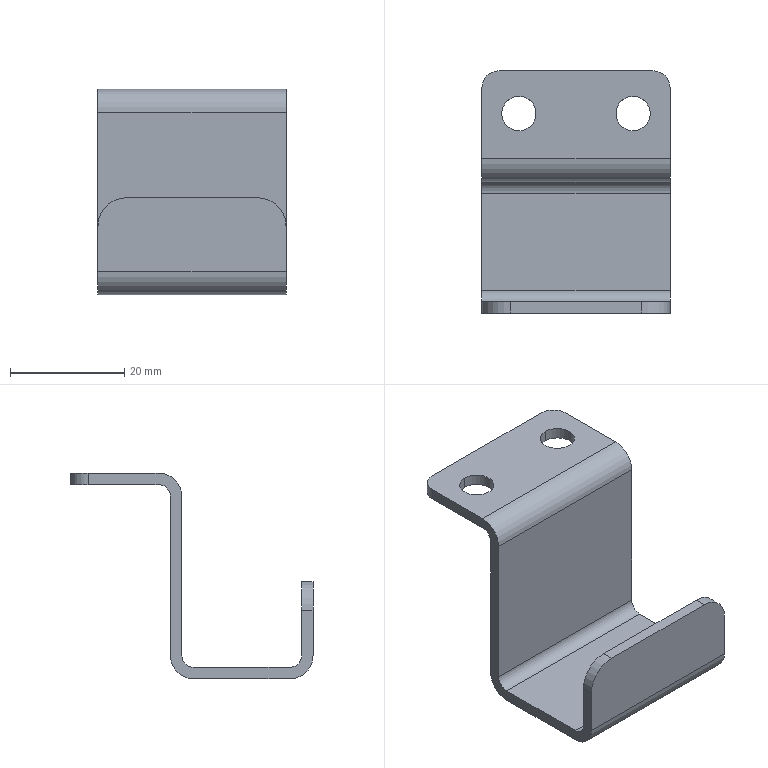Part | NX | features solid 2 | 1 solid | 26 faces | box 33 x 42.445 x 36 mm | volume 5638 mm3 | cylinder 14 | plane 12 | commonest cylinder face diameters 6 x6 4 x3 8 x3 10 x2
STEP:
#1=CARTESIAN_POINT('',(-461.,-1639.945,294.));
#2=VERTEX_POINT('',#1);
#3=CARTESIAN_POINT('',(-461.,-1637.945,296.));
#4=VERTEX_POINT('',#3);
#5=CARTESIAN_POINT('',(-461.,-1637.945,294.));
#6=DIRECTION('',(-1.,0.,0.));
#7=DIRECTION('',(0.,-1.,0.));
#8=AXIS2_PLACEMENT_3D('',#5,#6,#7);
#9=CIRCLE('',#8,2.);
#10=EDGE_CURVE('',#2,#4,#9,.T.);
#11=ORIENTED_EDGE('',*,*,#10,.F.);
#12=CARTESIAN_POINT('',(-494.,-1639.945,294.));
#13=VERTEX_POINT('',#12);
#14=CARTESIAN_POINT('',(-494.,-1639.945,294.));
#15=DIRECTION('',(1.,0.,0.));
#16=VECTOR('',#15,1000.);
#17=LINE('',#14,#16);
#18=EDGE_CURVE('',#13,#2,#17,.T.);
#19=ORIENTED_EDGE('',*,*,#18,.F.);
#20=CARTESIAN_POINT('',(-494.,-1637.945,296.));
#21=VERTEX_POINT('',#20);
#22=CARTESIAN_POINT('',(-494.,-1637.945,294.));
#23=DIRECTION('',(-1.,0.,0.));
#24=DIRECTION('',(0.,-1.,0.));
#25=AXIS2_PLACEMENT_3D('',#22,#23,#24);
#26=CIRCLE('',#25,2.);
#27=EDGE_CURVE('',#13,#21,#26,.T.);
#28=ORIENTED_EDGE('',*,*,#27,.T.);
#29=CARTESIAN_POINT('',(-494.,-1637.945,296.));
#30=DIRECTION('',(1.,0.,0.));
#31=VECTOR('',#30,1000.);
#32=LINE('',#29,#31);
#33=EDGE_CURVE('',#21,#4,#32,.T.);
#34=ORIENTED_EDGE('',*,*,#33,.T.);
#35=EDGE_LOOP('',(#11,#19,#28,#34));
#36=FACE_BOUND('',#35,.T.);
#37=CARTESIAN_POINT('',(-461.,-1637.945,294.));
#38=DIRECTION('',(-1.,0.,0.));
#39=DIRECTION('',(0.,1.,0.));
#40=AXIS2_PLACEMENT_3D('',#37,#38,#39);
#41=CYLINDRICAL_SURFACE('',#40,2.);
#42=ADVANCED_FACE('',(#36),#41,.F.);
#43=CARTESIAN_POINT('',(-461.,-1641.945,294.));
#44=VERTEX_POINT('',#43);
#45=CARTESIAN_POINT('',(-461.,-1637.945,298.));
#46=VERTEX_POINT('',#45);
#47=CARTESIAN_POINT('',(-461.,-1637.945,294.));
#48=DIRECTION('',(-1.,0.,0.));
#49=DIRECTION('',(0.,1.,0.));
#50=AXIS2_PLACEMENT_3D('',#47,#48,#49);
#51=CIRCLE('',#50,4.);
#52=EDGE_CURVE('',#44,#46,#51,.T.);
#53=ORIENTED_EDGE('',*,*,#52,.T.);
#54=CARTESIAN_POINT('',(-494.,-1637.945,298.));
#55=VERTEX_POINT('',#54);
#56=CARTESIAN_POINT('',(-494.,-1637.945,298.));
#57=DIRECTION('',(1.,0.,0.));
#58=VECTOR('',#57,1000.);
#59=LINE('',#56,#58);
#60=EDGE_CURVE('',#55,#46,#59,.T.);
#61=ORIENTED_EDGE('',*,*,#60,.F.);
#62=CARTESIAN_POINT('',(-494.,-1641.945,294.));
#63=VERTEX_POINT('',#62);
#64=CARTESIAN_POINT('',(-494.,-1637.945,294.));
#65=DIRECTION('',(-1.,0.,0.));
#66=DIRECTION('',(0.,1.,0.));
#67=AXIS2_PLACEMENT_3D('',#64,#65,#66);
#68=CIRCLE('',#67,4.);
#69=EDGE_CURVE('',#63,#55,#68,.T.);
#70=ORIENTED_EDGE('',*,*,#69,.F.);
#71=CARTESIAN_POINT('',(-494.,-1641.945,294.));
#72=DIRECTION('',(1.,0.,0.));
#73=VECTOR('',#72,1000.);
#74=LINE('',#71,#73);
#75=EDGE_CURVE('',#63,#44,#74,.T.);
#76=ORIENTED_EDGE('',*,*,#75,.T.);
#77=EDGE_LOOP('',(#53,#61,#70,#76));
#78=FACE_BOUND('',#77,.T.);
#79=CARTESIAN_POINT('',(-461.,-1637.945,294.));
#80=DIRECTION('',(-1.,0.,0.));
#81=DIRECTION('',(0.,1.,0.));
#82=AXIS2_PLACEMENT_3D('',#79,#80,#81);
#83=CYLINDRICAL_SURFACE('',#82,4.);
#84=ADVANCED_FACE('',(#78),#83,.T.);
#85=CARTESIAN_POINT('',(-467.5,-1627.,296.));
#86=VERTEX_POINT('',#85);
#87=CARTESIAN_POINT('',(-467.5,-1633.,296.));
#88=VERTEX_POINT('',#87);
#89=CARTESIAN_POINT('',(-467.5,-1630.,296.));
#90=DIRECTION('',(0.,0.,-1.));
#91=DIRECTION('',(0.,-1.,0.));
#92=AXIS2_PLACEMENT_3D('',#89,#90,#91);
#93=CIRCLE('',#92,3.);
#94=EDGE_CURVE('',#86,#88,#93,.T.);
#95=ORIENTED_EDGE('',*,*,#94,.F.);
#96=CARTESIAN_POINT('',(-467.5,-1630.,296.));
#97=DIRECTION('',(0.,0.,-1.));
#98=DIRECTION('',(0.,-1.,0.));
#99=AXIS2_PLACEMENT_3D('',#96,#97,#98);
#100=CIRCLE('',#99,3.);
#101=EDGE_CURVE('',#88,#86,#100,.T.);
#102=ORIENTED_EDGE('',*,*,#101,.F.);
#103=EDGE_LOOP('',(#95,#102));
#104=FACE_BOUND('',#103,.T.);
#105=CARTESIAN_POINT('',(-487.5,-1627.,296.));
#106=VERTEX_POINT('',#105);
#107=CARTESIAN_POINT('',(-487.5,-1633.,296.));
#108=VERTEX_POINT('',#107);
#109=CARTESIAN_POINT('',(-487.5,-1630.,296.));
#110=DIRECTION('',(0.,0.,-1.));
#111=DIRECTION('',(0.,-1.,0.));
#112=AXIS2_PLACEMENT_3D('',#109,#110,#111);
#113=CIRCLE('',#112,3.);
#114=EDGE_CURVE('',#106,#108,#113,.T.);
#115=ORIENTED_EDGE('',*,*,#114,.F.);
#116=CARTESIAN_POINT('',(-487.5,-1630.,296.));
#117=DIRECTION('',(0.,0.,-1.));
#118=DIRECTION('',(0.,-1.,0.));
#119=AXIS2_PLACEMENT_3D('',#116,#117,#118);
#120=CIRCLE('',#119,3.);
#121=EDGE_CURVE('',#108,#106,#120,.T.);
#122=ORIENTED_EDGE('',*,*,#121,.F.);
#123=EDGE_LOOP('',(#115,#122));
#124=FACE_BOUND('',#123,.T.);
#125=ORIENTED_EDGE('',*,*,#33,.F.);
#126=CARTESIAN_POINT('',(-494.,-1625.5,296.));
#127=VERTEX_POINT('',#126);
#128=CARTESIAN_POINT('',(-494.,-1622.5,296.));
#129=DIRECTION('',(0.,1.,0.));
#130=VECTOR('',#129,1000.);
#131=LINE('',#128,#130);
#132=EDGE_CURVE('',#21,#127,#131,.T.);
#133=ORIENTED_EDGE('',*,*,#132,.T.);
#134=CARTESIAN_POINT('',(-491.,-1622.5,296.));
#135=VERTEX_POINT('',#134);
#136=CARTESIAN_POINT('',(-491.,-1625.5,296.));
#137=DIRECTION('',(0.,0.,-1.));
#138=DIRECTION('',(0.,-1.,0.));
#139=AXIS2_PLACEMENT_3D('',#136,#137,#138);
#140=CIRCLE('',#139,3.);
#141=EDGE_CURVE('',#127,#135,#140,.T.);
#142=ORIENTED_EDGE('',*,*,#141,.T.);
#143=CARTESIAN_POINT('',(-464.,-1622.5,296.));
#144=VERTEX_POINT('',#143);
#145=CARTESIAN_POINT('',(-494.,-1622.5,296.));
#146=DIRECTION('',(1.,0.,0.));
#147=VECTOR('',#146,1000.);
#148=LINE('',#145,#147);
#149=EDGE_CURVE('',#135,#144,#148,.T.);
#150=ORIENTED_EDGE('',*,*,#149,.T.);
#151=CARTESIAN_POINT('',(-461.,-1625.5,296.));
#152=VERTEX_POINT('',#151);
#153=CARTESIAN_POINT('',(-464.,-1625.5,296.));
#154=DIRECTION('',(0.,0.,-1.));
#155=DIRECTION('',(0.,-1.,0.));
#156=AXIS2_PLACEMENT_3D('',#153,#154,#155);
#157=CIRCLE('',#156,3.);
#158=EDGE_CURVE('',#144,#152,#157,.T.);
#159=ORIENTED_EDGE('',*,*,#158,.T.);
#160=CARTESIAN_POINT('',(-461.,-1622.5,296.));
#161=DIRECTION('',(0.,1.,0.));
#162=VECTOR('',#161,1000.);
#163=LINE('',#160,#162);
#164=EDGE_CURVE('',#4,#152,#163,.T.);
#165=ORIENTED_EDGE('',*,*,#164,.F.);
#166=EDGE_LOOP('',(#125,#133,#142,#150,#159,#165));
#167=FACE_BOUND('',#166,.T.);
#168=CARTESIAN_POINT('',(-494.,-1622.5,296.));
#169=DIRECTION('',(0.,0.,-1.));
#170=DIRECTION('',(0.,-1.,0.));
#171=AXIS2_PLACEMENT_3D('',#168,#169,#170);
#172=PLANE('',#171);
#173=ADVANCED_FACE('',(#104,#124,#167),#172,.T.);
#174=CARTESIAN_POINT('',(-467.5,-1627.,298.));
#175=VERTEX_POINT('',#174);
#176=CARTESIAN_POINT('',(-467.5,-1633.,298.));
#177=VERTEX_POINT('',#176);
#178=CARTESIAN_POINT('',(-467.5,-1630.,298.));
#179=DIRECTION('',(0.,0.,1.));
#180=DIRECTION('',(1.,0.,0.));
#181=AXIS2_PLACEMENT_3D('',#178,#179,#180);
#182=CIRCLE('',#181,3.);
#183=EDGE_CURVE('',#175,#177,#182,.T.);
#184=ORIENTED_EDGE('',*,*,#183,.F.);
#185=CARTESIAN_POINT('',(-467.5,-1630.,298.));
#186=DIRECTION('',(0.,0.,1.));
#187=DIRECTION('',(1.,0.,0.));
#188=AXIS2_PLACEMENT_3D('',#185,#186,#187);
#189=CIRCLE('',#188,3.);
#190=EDGE_CURVE('',#177,#175,#189,.T.);
#191=ORIENTED_EDGE('',*,*,#190,.F.);
#192=EDGE_LOOP('',(#184,#191));
#193=FACE_BOUND('',#192,.T.);
#194=CARTESIAN_POINT('',(-487.5,-1627.,298.));
#195=VERTEX_POINT('',#194);
#196=CARTESIAN_POINT('',(-487.5,-1633.,298.));
#197=VERTEX_POINT('',#196);
#198=CARTESIAN_POINT('',(-487.5,-1630.,298.));
#199=DIRECTION('',(0.,0.,1.));
#200=DIRECTION('',(1.,0.,0.));
#201=AXIS2_PLACEMENT_3D('',#198,#199,#200);
#202=CIRCLE('',#201,3.);
#203=EDGE_CURVE('',#195,#197,#202,.T.);
#204=ORIENTED_EDGE('',*,*,#203,.F.);
#205=CARTESIAN_POINT('',(-487.5,-1630.,298.));
#206=DIRECTION('',(0.,0.,1.));
#207=DIRECTION('',(1.,0.,0.));
#208=AXIS2_PLACEMENT_3D('',#205,#206,#207);
#209=CIRCLE('',#208,3.);
#210=EDGE_CURVE('',#197,#195,#209,.T.);
#211=ORIENTED_EDGE('',*,*,#210,.F.);
#212=EDGE_LOOP('',(#204,#211));
#213=FACE_BOUND('',#212,.T.);
#214=CARTESIAN_POINT('',(-494.,-1625.5,298.));
#215=VERTEX_POINT('',#214);
#216=CARTESIAN_POINT('',(-494.,-1622.5,298.));
#217=DIRECTION('',(0.,1.,0.));
#218=VECTOR('',#217,1000.);
#219=LINE('',#216,#218);
#220=EDGE_CURVE('',#55,#215,#219,.T.);
#221=ORIENTED_EDGE('',*,*,#220,.F.);
#222=ORIENTED_EDGE('',*,*,#60,.T.);
#223=CARTESIAN_POINT('',(-461.,-1625.5,298.));
#224=VERTEX_POINT('',#223);
#225=CARTESIAN_POINT('',(-461.,-1622.5,298.));
#226=DIRECTION('',(0.,1.,0.));
#227=VECTOR('',#226,1000.);
#228=LINE('',#225,#227);
#229=EDGE_CURVE('',#46,#224,#228,.T.);
#230=ORIENTED_EDGE('',*,*,#229,.T.);
#231=CARTESIAN_POINT('',(-464.,-1622.5,298.));
#232=VERTEX_POINT('',#231);
#233=CARTESIAN_POINT('',(-464.,-1625.5,298.));
#234=DIRECTION('',(0.,0.,1.));
#235=DIRECTION('',(0.,-1.,0.));
#236=AXIS2_PLACEMENT_3D('',#233,#234,#235);
#237=CIRCLE('',#236,3.);
#238=EDGE_CURVE('',#224,#232,#237,.T.);
#239=ORIENTED_EDGE('',*,*,#238,.T.);
#240=CARTESIAN_POINT('',(-491.,-1622.5,298.));
#241=VERTEX_POINT('',#240);
#242=CARTESIAN_POINT('',(-494.,-1622.5,298.));
#243=DIRECTION('',(1.,0.,0.));
#244=VECTOR('',#243,1000.);
#245=LINE('',#242,#244);
#246=EDGE_CURVE('',#241,#232,#245,.T.);
#247=ORIENTED_EDGE('',*,*,#246,.F.);
#248=CARTESIAN_POINT('',(-491.,-1625.5,298.));
#249=DIRECTION('',(0.,0.,1.));
#250=DIRECTION('',(0.,-1.,0.));
#251=AXIS2_PLACEMENT_3D('',#248,#249,#250);
#252=CIRCLE('',#251,3.);
#253=EDGE_CURVE('',#241,#215,#252,.T.);
#254=ORIENTED_EDGE('',*,*,#253,.T.);
#255=EDGE_LOOP('',(#221,#222,#230,#239,#247,#254));
#256=FACE_BOUND('',#255,.T.);
#257=CARTESIAN_POINT('',(-494.,-1622.5,298.));
#258=DIRECTION('',(0.,0.,-1.));
#259=DIRECTION('',(0.,-1.,0.));
#260=AXIS2_PLACEMENT_3D('',#257,#258,#259);
#261=PLANE('',#260);
#262=ADVANCED_FACE('',(#193,#213,#256),#261,.F.);
#263=ORIENTED_EDGE('',*,*,#141,.F.);
#264=CARTESIAN_POINT('',(-494.,-1625.5,319.));
#265=DIRECTION('',(0.,0.,-1.));
#266=VECTOR('',#265,1000.);
#267=LINE('',#264,#266);
#268=EDGE_CURVE('',#215,#127,#267,.T.);
#269=ORIENTED_EDGE('',*,*,#268,.F.);
#270=ORIENTED_EDGE('',*,*,#253,.F.);
#271=CARTESIAN_POINT('',(-491.,-1622.5,298.));
#272=DIRECTION('',(0.,0.,1.));
#273=VECTOR('',#272,1000.);
#274=LINE('',#271,#273);
#275=EDGE_CURVE('',#135,#241,#274,.T.);
#276=ORIENTED_EDGE('',*,*,#275,.F.);
#277=EDGE_LOOP('',(#263,#269,#270,#276));
#278=FACE_BOUND('',#277,.T.);
#279=CARTESIAN_POINT('',(-491.,-1625.5,298.));
#280=DIRECTION('',(0.,0.,1.));
#281=DIRECTION('',(0.,1.,0.));
#282=AXIS2_PLACEMENT_3D('',#279,#280,#281);
#283=CYLINDRICAL_SURFACE('',#282,3.);
#284=ADVANCED_FACE('',(#278),#283,.T.);
#285=CARTESIAN_POINT('',(-487.5,-1633.,231.532));
#286=DIRECTION('',(0.,0.,1.));
#287=VECTOR('',#286,1000.);
#288=LINE('',#285,#287);
#289=EDGE_CURVE('',#197,#108,#288,.F.);
#290=ORIENTED_EDGE('',*,*,#289,.T.);
#291=ORIENTED_EDGE('',*,*,#121,.T.);
#292=CARTESIAN_POINT('',(-487.5,-1627.,231.532));
#293=DIRECTION('',(0.,0.,1.));
#294=VECTOR('',#293,1000.);
#295=LINE('',#292,#294);
#296=EDGE_CURVE('',#106,#195,#295,.T.);
#297=ORIENTED_EDGE('',*,*,#296,.T.);
#298=ORIENTED_EDGE('',*,*,#203,.T.);
#299=EDGE_LOOP('',(#290,#291,#297,#298));
#300=FACE_BOUND('',#299,.T.);
#301=CARTESIAN_POINT('',(-487.5,-1630.,231.532));
#302=DIRECTION('',(0.,0.,1.));
#303=DIRECTION('',(0.,1.,0.));
#304=AXIS2_PLACEMENT_3D('',#301,#302,#303);
#305=CYLINDRICAL_SURFACE('',#304,3.);
#306=ADVANCED_FACE('',(#300),#305,.F.);
#307=CARTESIAN_POINT('',(-467.5,-1633.,231.532));
#308=DIRECTION('',(0.,0.,1.));
#309=VECTOR('',#308,1000.);
#310=LINE('',#307,#309);
#311=EDGE_CURVE('',#177,#88,#310,.F.);
#312=ORIENTED_EDGE('',*,*,#311,.T.);
#313=ORIENTED_EDGE('',*,*,#101,.T.);
#314=CARTESIAN_POINT('',(-467.5,-1627.,231.532));
#315=DIRECTION('',(0.,0.,1.));
#316=VECTOR('',#315,1000.);
#317=LINE('',#314,#316);
#318=EDGE_CURVE('',#86,#175,#317,.T.);
#319=ORIENTED_EDGE('',*,*,#318,.T.);
#320=ORIENTED_EDGE('',*,*,#183,.T.);
#321=EDGE_LOOP('',(#312,#313,#319,#320));
#322=FACE_BOUND('',#321,.T.);
#323=CARTESIAN_POINT('',(-467.5,-1630.,231.532));
#324=DIRECTION('',(0.,0.,1.));
#325=DIRECTION('',(0.,1.,0.));
#326=AXIS2_PLACEMENT_3D('',#323,#324,#325);
#327=CYLINDRICAL_SURFACE('',#326,3.);
#328=ADVANCED_FACE('',(#322),#327,.F.);
#329=ORIENTED_EDGE('',*,*,#158,.F.);
#330=CARTESIAN_POINT('',(-464.,-1622.5,298.));
#331=DIRECTION('',(0.,0.,-1.));
#332=VECTOR('',#331,1000.);
#333=LINE('',#330,#332);
#334=EDGE_CURVE('',#232,#144,#333,.T.);
#335=ORIENTED_EDGE('',*,*,#334,.F.);
#336=ORIENTED_EDGE('',*,*,#238,.F.);
#337=CARTESIAN_POINT('',(-461.,-1625.5,317.));
#338=DIRECTION('',(0.,0.,1.));
#339=VECTOR('',#338,1000.);
#340=LINE('',#337,#339);
#341=EDGE_CURVE('',#152,#224,#340,.T.);
#342=ORIENTED_EDGE('',*,*,#341,.F.);
#343=EDGE_LOOP('',(#329,#335,#336,#342));
#344=FACE_BOUND('',#343,.T.);
#345=CARTESIAN_POINT('',(-464.,-1625.5,317.));
#346=DIRECTION('',(0.,0.,1.));
#347=DIRECTION('',(0.,1.,0.));
#348=AXIS2_PLACEMENT_3D('',#345,#346,#347);
#349=CYLINDRICAL_SURFACE('',#348,3.);
#350=ADVANCED_FACE('',(#344),#349,.T.);
#351=ORIENTED_EDGE('',*,*,#246,.T.);
#352=ORIENTED_EDGE('',*,*,#334,.T.);
#353=ORIENTED_EDGE('',*,*,#149,.F.);
#354=ORIENTED_EDGE('',*,*,#275,.T.);
#355=EDGE_LOOP('',(#351,#352,#353,#354));
#356=FACE_BOUND('',#355,.T.);
#357=CARTESIAN_POINT('',(-494.,-1622.5,298.));
#358=DIRECTION('',(0.,1.,0.));
#359=DIRECTION('',(1.,0.,0.));
#360=AXIS2_PLACEMENT_3D('',#357,#358,#359);
#361=PLANE('',#360);
#362=ADVANCED_FACE('',(#356),#361,.T.);
#363=CARTESIAN_POINT('',(-489.,-1664.945,279.));
#364=VERTEX_POINT('',#363);
#365=CARTESIAN_POINT('',(-494.,-1664.945,274.));
#366=VERTEX_POINT('',#365);
#367=CARTESIAN_POINT('',(-489.,-1664.945,274.));
#368=DIRECTION('',(0.,-1.,0.));
#369=DIRECTION('',(1.,0.,0.));
#370=AXIS2_PLACEMENT_3D('',#367,#368,#369);
#371=CIRCLE('',#370,5.);
#372=EDGE_CURVE('',#364,#366,#371,.T.);
#373=ORIENTED_EDGE('',*,*,#372,.F.);
#374=CARTESIAN_POINT('',(-489.,-1662.945,279.));
#375=VERTEX_POINT('',#374);
#376=CARTESIAN_POINT('',(-489.,-1662.945,279.));
#377=DIRECTION('',(0.,-1.,0.));
#378=VECTOR('',#377,1000.);
#379=LINE('',#376,#378);
#380=EDGE_CURVE('',#375,#364,#379,.T.);
#381=ORIENTED_EDGE('',*,*,#380,.F.);
#382=CARTESIAN_POINT('',(-494.,-1662.945,274.));
#383=VERTEX_POINT('',#382);
#384=CARTESIAN_POINT('',(-489.,-1662.945,274.));
#385=DIRECTION('',(0.,1.,0.));
#386=DIRECTION('',(1.,0.,0.));
#387=AXIS2_PLACEMENT_3D('',#384,#385,#386);
#388=CIRCLE('',#387,5.);
#389=EDGE_CURVE('',#383,#375,#388,.T.);
#390=ORIENTED_EDGE('',*,*,#389,.F.);
#391=CARTESIAN_POINT('',(-494.,-1662.945,274.));
#392=DIRECTION('',(0.,1.,0.));
#393=VECTOR('',#392,1000.);
#394=LINE('',#391,#393);
#395=EDGE_CURVE('',#366,#383,#394,.T.);
#396=ORIENTED_EDGE('',*,*,#395,.F.);
#397=EDGE_LOOP('',(#373,#381,#390,#396));
#398=FACE_BOUND('',#397,.T.);
#399=CARTESIAN_POINT('',(-489.,-1662.945,274.));
#400=DIRECTION('',(0.,-1.,0.));
#401=DIRECTION('',(1.,0.,0.));
#402=AXIS2_PLACEMENT_3D('',#399,#400,#401);
#403=CYLINDRICAL_SURFACE('',#402,5.);
#404=ADVANCED_FACE('',(#398),#403,.T.);
#405=CARTESIAN_POINT('',(-461.,-1664.945,274.));
#406=VERTEX_POINT('',#405);
#407=CARTESIAN_POINT('',(-466.,-1664.945,279.));
#408=VERTEX_POINT('',#407);
#409=CARTESIAN_POINT('',(-466.,-1664.945,274.));
#410=DIRECTION('',(0.,-1.,0.));
#411=DIRECTION('',(1.,0.,0.));
#412=AXIS2_PLACEMENT_3D('',#409,#410,#411);
#413=CIRCLE('',#412,5.);
#414=EDGE_CURVE('',#406,#408,#413,.T.);
#415=ORIENTED_EDGE('',*,*,#414,.F.);
#416=CARTESIAN_POINT('',(-461.,-1662.945,274.));
#417=VERTEX_POINT('',#416);
#418=CARTESIAN_POINT('',(-461.,-1660.945,274.));
#419=DIRECTION('',(0.,-1.,0.));
#420=VECTOR('',#419,1000.);
#421=LINE('',#418,#420);
#422=EDGE_CURVE('',#417,#406,#421,.T.);
#423=ORIENTED_EDGE('',*,*,#422,.F.);
#424=CARTESIAN_POINT('',(-466.,-1662.945,279.));
#425=VERTEX_POINT('',#424);
#426=CARTESIAN_POINT('',(-466.,-1662.945,274.));
#427=DIRECTION('',(0.,1.,0.));
#428=DIRECTION('',(1.,0.,0.));
#429=AXIS2_PLACEMENT_3D('',#426,#427,#428);
#430=CIRCLE('',#429,5.);
#431=EDGE_CURVE('',#425,#417,#430,.T.);
#432=ORIENTED_EDGE('',*,*,#431,.F.);
#433=CARTESIAN_POINT('',(-466.,-1662.945,279.));
#434=DIRECTION('',(0.,1.,0.));
#435=VECTOR('',#434,1000.);
#436=LINE('',#433,#435);
#437=EDGE_CURVE('',#408,#425,#436,.T.);
#438=ORIENTED_EDGE('',*,*,#437,.F.);
#439=EDGE_LOOP('',(#415,#423,#432,#438));
#440=FACE_BOUND('',#439,.T.);
#441=CARTESIAN_POINT('',(-466.,-1662.945,274.));
#442=DIRECTION('',(0.,-1.,0.));
#443=DIRECTION('',(1.,0.,0.));
#444=AXIS2_PLACEMENT_3D('',#441,#442,#443);
#445=CYLINDRICAL_SURFACE('',#444,5.);
#446=ADVANCED_FACE('',(#440),#445,.T.);
#447=CARTESIAN_POINT('',(-461.,-1643.945,262.));
#448=VERTEX_POINT('',#447);
#449=CARTESIAN_POINT('',(-461.,-1639.945,266.));
#450=VERTEX_POINT('',#449);
#451=CARTESIAN_POINT('',(-461.,-1643.945,266.));
#452=DIRECTION('',(1.,0.,0.));
#453=DIRECTION('',(0.,1.,0.));
#454=AXIS2_PLACEMENT_3D('',#451,#452,#453);
#455=CIRCLE('',#454,4.);
#456=EDGE_CURVE('',#448,#450,#455,.T.);
#457=ORIENTED_EDGE('',*,*,#456,.F.);
#458=CARTESIAN_POINT('',(-494.,-1643.945,262.));
#459=VERTEX_POINT('',#458);
#460=CARTESIAN_POINT('',(-494.,-1643.945,262.));
#461=DIRECTION('',(1.,0.,0.));
#462=VECTOR('',#461,1000.);
#463=LINE('',#460,#462);
#464=EDGE_CURVE('',#459,#448,#463,.T.);
#465=ORIENTED_EDGE('',*,*,#464,.F.);
#466=CARTESIAN_POINT('',(-494.,-1639.945,266.));
#467=VERTEX_POINT('',#466);
#468=CARTESIAN_POINT('',(-494.,-1643.945,266.));
#469=DIRECTION('',(1.,0.,0.));
#470=DIRECTION('',(0.,1.,0.));
#471=AXIS2_PLACEMENT_3D('',#468,#469,#470);
#472=CIRCLE('',#471,4.);
#473=EDGE_CURVE('',#459,#467,#472,.T.);
#474=ORIENTED_EDGE('',*,*,#473,.T.);
#475=CARTESIAN_POINT('',(-494.,-1639.945,266.));
#476=DIRECTION('',(1.,0.,0.));
#477=VECTOR('',#476,1000.);
#478=LINE('',#475,#477);
#479=EDGE_CURVE('',#467,#450,#478,.T.);
#480=ORIENTED_EDGE('',*,*,#479,.T.);
#481=EDGE_LOOP('',(#457,#465,#474,#480));
#482=FACE_BOUND('',#481,.T.);
#483=CARTESIAN_POINT('',(-494.,-1643.945,266.));
#484=DIRECTION('',(1.,0.,0.));
#485=DIRECTION('',(0.,1.,0.));
#486=AXIS2_PLACEMENT_3D('',#483,#484,#485);
#487=CYLINDRICAL_SURFACE('',#486,4.);
#488=ADVANCED_FACE('',(#482),#487,.T.);
#489=CARTESIAN_POINT('',(-461.,-1660.945,262.));
#490=VERTEX_POINT('',#489);
#491=CARTESIAN_POINT('',(-461.,-1641.945,262.));
#492=DIRECTION('',(0.,1.,0.));
#493=VECTOR('',#492,1000.);
#494=LINE('',#491,#493);
#495=EDGE_CURVE('',#490,#448,#494,.T.);
#496=ORIENTED_EDGE('',*,*,#495,.F.);
#497=CARTESIAN_POINT('',(-494.,-1660.945,262.));
#498=VERTEX_POINT('',#497);
#499=CARTESIAN_POINT('',(-494.,-1660.945,262.));
#500=DIRECTION('',(1.,0.,0.));
#501=VECTOR('',#500,1000.);
#502=LINE('',#499,#501);
#503=EDGE_CURVE('',#498,#490,#502,.T.);
#504=ORIENTED_EDGE('',*,*,#503,.F.);
#505=CARTESIAN_POINT('',(-494.,-1641.945,262.));
#506=DIRECTION('',(0.,1.,0.));
#507=VECTOR('',#506,1000.);
#508=LINE('',#505,#507);
#509=EDGE_CURVE('',#498,#459,#508,.T.);
#510=ORIENTED_EDGE('',*,*,#509,.T.);
#511=ORIENTED_EDGE('',*,*,#464,.T.);
#512=EDGE_LOOP('',(#496,#504,#510,#511));
#513=FACE_BOUND('',#512,.T.);
#514=CARTESIAN_POINT('',(-494.,-1641.945,262.));
#515=DIRECTION('',(0.,0.,-1.));
#516=DIRECTION('',(0.,-1.,0.));
#517=AXIS2_PLACEMENT_3D('',#514,#515,#516);
#518=PLANE('',#517);
#519=ADVANCED_FACE('',(#513),#518,.T.);
#520=CARTESIAN_POINT('',(-461.,-1664.945,266.));
#521=VERTEX_POINT('',#520);
#522=CARTESIAN_POINT('',(-461.,-1660.945,266.));
#523=DIRECTION('',(1.,0.,0.));
#524=DIRECTION('',(0.,1.,0.));
#525=AXIS2_PLACEMENT_3D('',#522,#523,#524);
#526=CIRCLE('',#525,4.);
#527=EDGE_CURVE('',#521,#490,#526,.T.);
#528=ORIENTED_EDGE('',*,*,#527,.F.);
#529=CARTESIAN_POINT('',(-494.,-1664.945,266.));
#530=VERTEX_POINT('',#529);
#531=CARTESIAN_POINT('',(-494.,-1664.945,266.));
#532=DIRECTION('',(1.,0.,0.));
#533=VECTOR('',#532,1000.);
#534=LINE('',#531,#533);
#535=EDGE_CURVE('',#530,#521,#534,.T.);
#536=ORIENTED_EDGE('',*,*,#535,.F.);
#537=CARTESIAN_POINT('',(-494.,-1660.945,266.));
#538=DIRECTION('',(1.,0.,0.));
#539=DIRECTION('',(0.,1.,0.));
#540=AXIS2_PLACEMENT_3D('',#537,#538,#539);
#541=CIRCLE('',#540,4.);
#542=EDGE_CURVE('',#530,#498,#541,.T.);
#543=ORIENTED_EDGE('',*,*,#542,.T.);
#544=ORIENTED_EDGE('',*,*,#503,.T.);
#545=EDGE_LOOP('',(#528,#536,#543,#544));
#546=FACE_BOUND('',#545,.T.);
#547=CARTESIAN_POINT('',(-494.,-1660.945,266.));
#548=DIRECTION('',(1.,0.,0.));
#549=DIRECTION('',(0.,1.,0.));
#550=AXIS2_PLACEMENT_3D('',#547,#548,#549);
#551=CYLINDRICAL_SURFACE('',#550,4.);
#552=ADVANCED_FACE('',(#546),#551,.T.);
#553=CARTESIAN_POINT('',(-461.,-1664.945,264.));
#554=DIRECTION('',(0.,0.,-1.));
#555=VECTOR('',#554,1000.);
#556=LINE('',#553,#555);
#557=EDGE_CURVE('',#406,#521,#556,.T.);
#558=ORIENTED_EDGE('',*,*,#557,.F.);
#559=ORIENTED_EDGE('',*,*,#414,.T.);
#560=CARTESIAN_POINT('',(-494.,-1664.945,279.));
#561=DIRECTION('',(1.,0.,0.));
#562=VECTOR('',#561,1000.);
#563=LINE('',#560,#562);
#564=EDGE_CURVE('',#364,#408,#563,.T.);
#565=ORIENTED_EDGE('',*,*,#564,.F.);
#566=ORIENTED_EDGE('',*,*,#372,.T.);
#567=CARTESIAN_POINT('',(-494.,-1664.945,264.));
#568=DIRECTION('',(0.,0.,-1.));
#569=VECTOR('',#568,1000.);
#570=LINE('',#567,#569);
#571=EDGE_CURVE('',#366,#530,#570,.T.);
#572=ORIENTED_EDGE('',*,*,#571,.T.);
#573=ORIENTED_EDGE('',*,*,#535,.T.);
#574=EDGE_LOOP('',(#558,#559,#565,#566,#572,#573));
#575=FACE_BOUND('',#574,.T.);
#576=CARTESIAN_POINT('',(-494.,-1664.945,264.));
#577=DIRECTION('',(0.,-1.,0.));
#578=DIRECTION('',(0.,0.,-1.));
#579=AXIS2_PLACEMENT_3D('',#576,#577,#578);
#580=PLANE('',#579);
#581=ADVANCED_FACE('',(#575),#580,.T.);
#582=ORIENTED_EDGE('',*,*,#75,.F.);
#583=CARTESIAN_POINT('',(-494.,-1641.945,266.));
#584=VERTEX_POINT('',#583);
#585=CARTESIAN_POINT('',(-494.,-1641.945,314.));
#586=DIRECTION('',(0.,0.,1.));
#587=VECTOR('',#586,1000.);
#588=LINE('',#585,#587);
#589=EDGE_CURVE('',#584,#63,#588,.T.);
#590=ORIENTED_EDGE('',*,*,#589,.F.);
#591=CARTESIAN_POINT('',(-461.,-1641.945,266.));
#592=VERTEX_POINT('',#591);
#593=CARTESIAN_POINT('',(-494.,-1641.945,266.));
#594=DIRECTION('',(1.,0.,0.));
#595=VECTOR('',#594,1000.);
#596=LINE('',#593,#595);
#597=EDGE_CURVE('',#584,#592,#596,.T.);
#598=ORIENTED_EDGE('',*,*,#597,.T.);
#599=CARTESIAN_POINT('',(-461.,-1641.945,314.));
#600=DIRECTION('',(0.,0.,1.));
#601=VECTOR('',#600,1000.);
#602=LINE('',#599,#601);
#603=EDGE_CURVE('',#592,#44,#602,.T.);
#604=ORIENTED_EDGE('',*,*,#603,.T.);
#605=EDGE_LOOP('',(#582,#590,#598,#604));
#606=FACE_BOUND('',#605,.T.);
#607=CARTESIAN_POINT('',(-494.,-1641.945,314.));
#608=DIRECTION('',(0.,1.,0.));
#609=DIRECTION('',(1.,0.,0.));
#610=AXIS2_PLACEMENT_3D('',#607,#608,#609);
#611=PLANE('',#610);
#612=ADVANCED_FACE('',(#606),#611,.F.);
#613=CARTESIAN_POINT('',(-461.,-1643.945,264.));
#614=VERTEX_POINT('',#613);
#615=CARTESIAN_POINT('',(-461.,-1643.945,266.));
#616=DIRECTION('',(1.,0.,0.));
#617=DIRECTION('',(0.,-1.,0.));
#618=AXIS2_PLACEMENT_3D('',#615,#616,#617);
#619=CIRCLE('',#618,2.);
#620=EDGE_CURVE('',#614,#592,#619,.T.);
#621=ORIENTED_EDGE('',*,*,#620,.T.);
#622=ORIENTED_EDGE('',*,*,#597,.F.);
#623=CARTESIAN_POINT('',(-494.,-1643.945,264.));
#624=VERTEX_POINT('',#623);
#625=CARTESIAN_POINT('',(-494.,-1643.945,266.));
#626=DIRECTION('',(1.,0.,0.));
#627=DIRECTION('',(0.,-1.,0.));
#628=AXIS2_PLACEMENT_3D('',#625,#626,#627);
#629=CIRCLE('',#628,2.);
#630=EDGE_CURVE('',#624,#584,#629,.T.);
#631=ORIENTED_EDGE('',*,*,#630,.F.);
#632=CARTESIAN_POINT('',(-494.,-1643.945,264.));
#633=DIRECTION('',(1.,0.,0.));
#634=VECTOR('',#633,1000.);
#635=LINE('',#632,#634);
#636=EDGE_CURVE('',#624,#614,#635,.T.);
#637=ORIENTED_EDGE('',*,*,#636,.T.);
#638=EDGE_LOOP('',(#621,#622,#631,#637));
#639=FACE_BOUND('',#638,.T.);
#640=CARTESIAN_POINT('',(-494.,-1643.945,266.));
#641=DIRECTION('',(1.,0.,0.));
#642=DIRECTION('',(0.,1.,0.));
#643=AXIS2_PLACEMENT_3D('',#640,#641,#642);
#644=CYLINDRICAL_SURFACE('',#643,2.);
#645=ADVANCED_FACE('',(#639),#644,.F.);
#646=CARTESIAN_POINT('',(-461.,-1660.945,264.));
#647=VERTEX_POINT('',#646);
#648=CARTESIAN_POINT('',(-461.,-1641.945,264.));
#649=DIRECTION('',(0.,1.,0.));
#650=VECTOR('',#649,1000.);
#651=LINE('',#648,#650);
#652=EDGE_CURVE('',#647,#614,#651,.T.);
#653=ORIENTED_EDGE('',*,*,#652,.T.);
#654=ORIENTED_EDGE('',*,*,#636,.F.);
#655=CARTESIAN_POINT('',(-494.,-1660.945,264.));
#656=VERTEX_POINT('',#655);
#657=CARTESIAN_POINT('',(-494.,-1641.945,264.));
#658=DIRECTION('',(0.,1.,0.));
#659=VECTOR('',#658,1000.);
#660=LINE('',#657,#659);
#661=EDGE_CURVE('',#656,#624,#660,.T.);
#662=ORIENTED_EDGE('',*,*,#661,.F.);
#663=CARTESIAN_POINT('',(-494.,-1660.945,264.));
#664=DIRECTION('',(1.,0.,0.));
#665=VECTOR('',#664,1000.);
#666=LINE('',#663,#665);
#667=EDGE_CURVE('',#656,#647,#666,.T.);
#668=ORIENTED_EDGE('',*,*,#667,.T.);
#669=EDGE_LOOP('',(#653,#654,#662,#668));
#670=FACE_BOUND('',#669,.T.);
#671=CARTESIAN_POINT('',(-494.,-1641.945,264.));
#672=DIRECTION('',(0.,0.,-1.));
#673=DIRECTION('',(0.,-1.,0.));
#674=AXIS2_PLACEMENT_3D('',#671,#672,#673);
#675=PLANE('',#674);
#676=ADVANCED_FACE('',(#670),#675,.F.);
#677=CARTESIAN_POINT('',(-461.,-1662.945,266.));
#678=VERTEX_POINT('',#677);
#679=CARTESIAN_POINT('',(-461.,-1660.945,266.));
#680=DIRECTION('',(1.,0.,0.));
#681=DIRECTION('',(0.,-1.,0.));
#682=AXIS2_PLACEMENT_3D('',#679,#680,#681);
#683=CIRCLE('',#682,2.);
#684=EDGE_CURVE('',#678,#647,#683,.T.);
#685=ORIENTED_EDGE('',*,*,#684,.T.);
#686=ORIENTED_EDGE('',*,*,#667,.F.);
#687=CARTESIAN_POINT('',(-494.,-1662.945,266.));
#688=VERTEX_POINT('',#687);
#689=CARTESIAN_POINT('',(-494.,-1660.945,266.));
#690=DIRECTION('',(1.,0.,0.));
#691=DIRECTION('',(0.,-1.,0.));
#692=AXIS2_PLACEMENT_3D('',#689,#690,#691);
#693=CIRCLE('',#692,2.);
#694=EDGE_CURVE('',#688,#656,#693,.T.);
#695=ORIENTED_EDGE('',*,*,#694,.F.);
#696=CARTESIAN_POINT('',(-494.,-1662.945,266.));
#697=DIRECTION('',(1.,0.,0.));
#698=VECTOR('',#697,1000.);
#699=LINE('',#696,#698);
#700=EDGE_CURVE('',#688,#678,#699,.T.);
#701=ORIENTED_EDGE('',*,*,#700,.T.);
#702=EDGE_LOOP('',(#685,#686,#695,#701));
#703=FACE_BOUND('',#702,.T.);
#704=CARTESIAN_POINT('',(-494.,-1660.945,266.));
#705=DIRECTION('',(1.,0.,0.));
#706=DIRECTION('',(0.,1.,0.));
#707=AXIS2_PLACEMENT_3D('',#704,#705,#706);
#708=CYLINDRICAL_SURFACE('',#707,2.);
#709=ADVANCED_FACE('',(#703),#708,.F.);
#710=CARTESIAN_POINT('',(-494.,-1662.945,279.));
#711=DIRECTION('',(1.,0.,0.));
#712=VECTOR('',#711,1000.);
#713=LINE('',#710,#712);
#714=EDGE_CURVE('',#375,#425,#713,.T.);
#715=ORIENTED_EDGE('',*,*,#714,.T.);
#716=ORIENTED_EDGE('',*,*,#431,.T.);
#717=CARTESIAN_POINT('',(-461.,-1662.945,264.));
#718=DIRECTION('',(0.,0.,-1.));
#719=VECTOR('',#718,1000.);
#720=LINE('',#717,#719);
#721=EDGE_CURVE('',#417,#678,#720,.T.);
#722=ORIENTED_EDGE('',*,*,#721,.T.);
#723=ORIENTED_EDGE('',*,*,#700,.F.);
#724=CARTESIAN_POINT('',(-494.,-1662.945,264.));
#725=DIRECTION('',(0.,0.,-1.));
#726=VECTOR('',#725,1000.);
#727=LINE('',#724,#726);
#728=EDGE_CURVE('',#383,#688,#727,.T.);
#729=ORIENTED_EDGE('',*,*,#728,.F.);
#730=ORIENTED_EDGE('',*,*,#389,.T.);
#731=EDGE_LOOP('',(#715,#716,#722,#723,#729,#730));
#732=FACE_BOUND('',#731,.T.);
#733=CARTESIAN_POINT('',(-494.,-1662.945,264.));
#734=DIRECTION('',(0.,-1.,0.));
#735=DIRECTION('',(0.,0.,-1.));
#736=AXIS2_PLACEMENT_3D('',#733,#734,#735);
#737=PLANE('',#736);
#738=ADVANCED_FACE('',(#732),#737,.F.);
#739=CARTESIAN_POINT('',(-461.,-1639.945,314.));
#740=DIRECTION('',(0.,0.,1.));
#741=VECTOR('',#740,1000.);
#742=LINE('',#739,#741);
#743=EDGE_CURVE('',#450,#2,#742,.T.);
#744=ORIENTED_EDGE('',*,*,#743,.T.);
#745=ORIENTED_EDGE('',*,*,#10,.T.);
#746=ORIENTED_EDGE('',*,*,#164,.T.);
#747=ORIENTED_EDGE('',*,*,#341,.T.);
#748=ORIENTED_EDGE('',*,*,#229,.F.);
#749=ORIENTED_EDGE('',*,*,#52,.F.);
#750=ORIENTED_EDGE('',*,*,#603,.F.);
#751=ORIENTED_EDGE('',*,*,#620,.F.);
#752=ORIENTED_EDGE('',*,*,#652,.F.);
#753=ORIENTED_EDGE('',*,*,#684,.F.);
#754=ORIENTED_EDGE('',*,*,#721,.F.);
#755=ORIENTED_EDGE('',*,*,#422,.T.);
#756=ORIENTED_EDGE('',*,*,#557,.T.);
#757=ORIENTED_EDGE('',*,*,#527,.T.);
#758=ORIENTED_EDGE('',*,*,#495,.T.);
#759=ORIENTED_EDGE('',*,*,#456,.T.);
#760=EDGE_LOOP('',(#744,#745,#746,#747,#748,#749,#750,#751,#752,#753,#754,#755,#756,#757,#758,#759));
#761=FACE_BOUND('',#760,.T.);
#762=CARTESIAN_POINT('',(-461.,-1660.945,266.));
#763=DIRECTION('',(1.,0.,0.));
#764=DIRECTION('',(0.,1.,0.));
#765=AXIS2_PLACEMENT_3D('',#762,#763,#764);
#766=PLANE('',#765);
#767=ADVANCED_FACE('',(#761),#766,.T.);
#768=ORIENTED_EDGE('',*,*,#564,.T.);
#769=ORIENTED_EDGE('',*,*,#437,.T.);
#770=ORIENTED_EDGE('',*,*,#714,.F.);
#771=ORIENTED_EDGE('',*,*,#380,.T.);
#772=EDGE_LOOP('',(#768,#769,#770,#771));
#773=FACE_BOUND('',#772,.T.);
#774=CARTESIAN_POINT('',(-494.,-1662.945,279.));
#775=DIRECTION('',(0.,0.,-1.));
#776=DIRECTION('',(0.,-1.,0.));
#777=AXIS2_PLACEMENT_3D('',#774,#775,#776);
#778=PLANE('',#777);
#779=ADVANCED_FACE('',(#773),#778,.F.);
#780=CARTESIAN_POINT('',(-494.,-1639.945,314.));
#781=DIRECTION('',(0.,0.,1.));
#782=VECTOR('',#781,1000.);
#783=LINE('',#780,#782);
#784=EDGE_CURVE('',#467,#13,#783,.T.);
#785=ORIENTED_EDGE('',*,*,#784,.T.);
#786=ORIENTED_EDGE('',*,*,#18,.T.);
#787=ORIENTED_EDGE('',*,*,#743,.F.);
#788=ORIENTED_EDGE('',*,*,#479,.F.);
#789=EDGE_LOOP('',(#785,#786,#787,#788));
#790=FACE_BOUND('',#789,.T.);
#791=CARTESIAN_POINT('',(-494.,-1639.945,314.));
#792=DIRECTION('',(0.,1.,0.));
#793=DIRECTION('',(1.,0.,0.));
#794=AXIS2_PLACEMENT_3D('',#791,#792,#793);
#795=PLANE('',#794);
#796=ADVANCED_FACE('',(#790),#795,.T.);
#797=ORIENTED_EDGE('',*,*,#589,.T.);
#798=ORIENTED_EDGE('',*,*,#69,.T.);
#799=ORIENTED_EDGE('',*,*,#220,.T.);
#800=ORIENTED_EDGE('',*,*,#268,.T.);
#801=ORIENTED_EDGE('',*,*,#132,.F.);
#802=ORIENTED_EDGE('',*,*,#27,.F.);
#803=ORIENTED_EDGE('',*,*,#784,.F.);
#804=ORIENTED_EDGE('',*,*,#473,.F.);
#805=ORIENTED_EDGE('',*,*,#509,.F.);
#806=ORIENTED_EDGE('',*,*,#542,.F.);
#807=ORIENTED_EDGE('',*,*,#571,.F.);
#808=ORIENTED_EDGE('',*,*,#395,.T.);
#809=ORIENTED_EDGE('',*,*,#728,.T.);
#810=ORIENTED_EDGE('',*,*,#694,.T.);
#811=ORIENTED_EDGE('',*,*,#661,.T.);
#812=ORIENTED_EDGE('',*,*,#630,.T.);
#813=EDGE_LOOP('',(#797,#798,#799,#800,#801,#802,#803,#804,#805,#806,#807,#808,#809,#810,#811,#812));
#814=FACE_BOUND('',#813,.T.);
#815=CARTESIAN_POINT('',(-494.,-1662.945,264.));
#816=DIRECTION('',(-1.,0.,0.));
#817=DIRECTION('',(0.,1.,0.));
#818=AXIS2_PLACEMENT_3D('',#815,#816,#817);
#819=PLANE('',#818);
#820=ADVANCED_FACE('',(#814),#819,.T.);
#821=ORIENTED_EDGE('',*,*,#94,.T.);
#822=ORIENTED_EDGE('',*,*,#311,.F.);
#823=ORIENTED_EDGE('',*,*,#190,.T.);
#824=ORIENTED_EDGE('',*,*,#318,.F.);
#825=EDGE_LOOP('',(#821,#822,#823,#824));
#826=FACE_BOUND('',#825,.T.);
#827=CARTESIAN_POINT('',(-467.5,-1630.,231.532));
#828=DIRECTION('',(0.,0.,1.));
#829=DIRECTION('',(0.,1.,0.));
#830=AXIS2_PLACEMENT_3D('',#827,#828,#829);
#831=CYLINDRICAL_SURFACE('',#830,3.);
#832=ADVANCED_FACE('',(#826),#831,.F.);
#833=ORIENTED_EDGE('',*,*,#114,.T.);
#834=ORIENTED_EDGE('',*,*,#289,.F.);
#835=ORIENTED_EDGE('',*,*,#210,.T.);
#836=ORIENTED_EDGE('',*,*,#296,.F.);
#837=EDGE_LOOP('',(#833,#834,#835,#836));
#838=FACE_BOUND('',#837,.T.);
#839=CARTESIAN_POINT('',(-487.5,-1630.,231.532));
#840=DIRECTION('',(0.,0.,1.));
#841=DIRECTION('',(0.,1.,0.));
#842=AXIS2_PLACEMENT_3D('',#839,#840,#841);
#843=CYLINDRICAL_SURFACE('',#842,3.);
#844=ADVANCED_FACE('',(#838),#843,.F.);
#845=CLOSED_SHELL('',(#42,#84,#173,#262,#284,#306,#328,#350,#362,#404,#446,#488,#519,#552,#581,#612,#645,#676,#709,#738,#767,#779,#796,#820,#832,#844));
#846=MANIFOLD_SOLID_BREP('',#845);
#847=(LENGTH_UNIT()NAMED_UNIT(*)SI_UNIT(.MILLI.,.METRE.));
#848=UNCERTAINTY_MEASURE_WITH_UNIT(LENGTH_MEASURE(0.00001),#847,'','');
#849=(NAMED_UNIT(*)PLANE_ANGLE_UNIT()SI_UNIT($,.RADIAN.));
#850=(NAMED_UNIT(*)SI_UNIT($,.STERADIAN.)SOLID_ANGLE_UNIT());
#851=(GEOMETRIC_REPRESENTATION_CONTEXT(3)GLOBAL_UNCERTAINTY_ASSIGNED_CONTEXT((#848))GLOBAL_UNIT_ASSIGNED_CONTEXT((#847,#849,#850))REPRESENTATION_CONTEXT('',''));
#852=ADVANCED_BREP_SHAPE_REPRESENTATION('',(#846),#851);